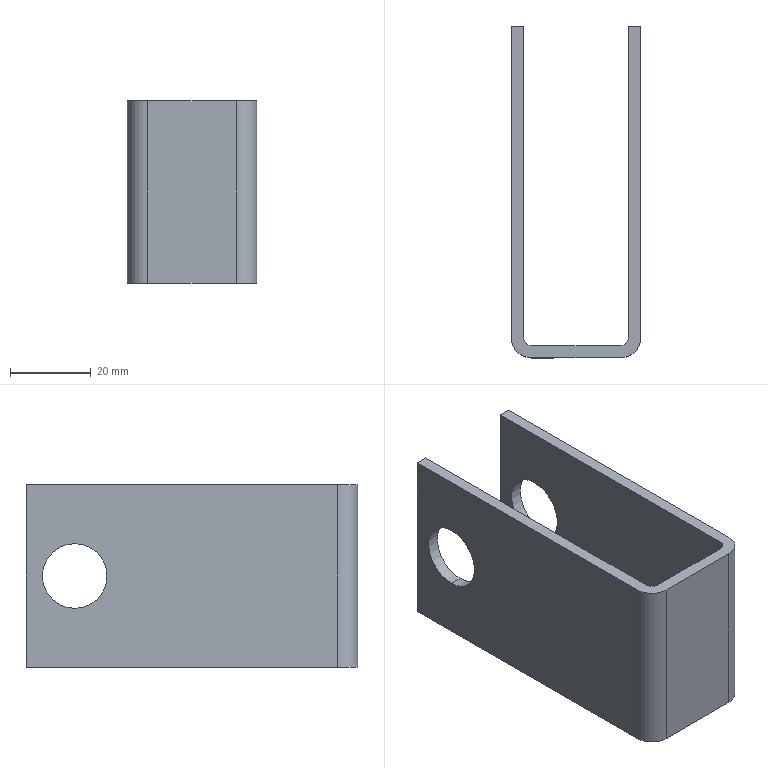Part | SolidWorks | features Extrusion 1, ICE 1 | 1 solid | 18 faces | box 32 x 82 x 45 mm | volume 24038 mm3 | plane 10 | cylinder 8 | commonest cylinder face diameters 16 x4 4 x2 10 x2
STEP:
#1=CARTESIAN_POINT('',(29.,-12.,30.5));
#2=VERTEX_POINT('',#1);
#3=CARTESIAN_POINT('',(29.,-12.,14.5));
#4=VERTEX_POINT('',#3);
#5=CARTESIAN_POINT('',(29.,-12.,22.5));
#6=DIRECTION('',(1.,0.,0.));
#7=DIRECTION('',(0.,1.,0.));
#8=AXIS2_PLACEMENT_3D('',#5,#6,#7);
#9=CIRCLE('',#8,8.);
#10=EDGE_CURVE('',#2,#4,#9,.T.);
#11=ORIENTED_EDGE('',*,*,#10,.F.);
#12=CARTESIAN_POINT('',(32.,-12.,30.5));
#13=VERTEX_POINT('',#12);
#14=CARTESIAN_POINT('',(0.,-12.,30.5));
#15=DIRECTION('',(1.,0.,0.));
#16=VECTOR('',#15,1000.);
#17=LINE('',#14,#16);
#18=EDGE_CURVE('',#2,#13,#17,.T.);
#19=ORIENTED_EDGE('',*,*,#18,.T.);
#20=CARTESIAN_POINT('',(32.,-12.,14.5));
#21=VERTEX_POINT('',#20);
#22=CARTESIAN_POINT('',(32.,-12.,22.5));
#23=DIRECTION('',(1.,0.,0.));
#24=DIRECTION('',(0.,0.,-1.));
#25=AXIS2_PLACEMENT_3D('',#22,#23,#24);
#26=CIRCLE('',#25,8.);
#27=EDGE_CURVE('',#13,#21,#26,.T.);
#28=ORIENTED_EDGE('',*,*,#27,.T.);
#29=CARTESIAN_POINT('',(0.,-12.,14.5));
#30=DIRECTION('',(1.,0.,0.));
#31=VECTOR('',#30,1000.);
#32=LINE('',#29,#31);
#33=EDGE_CURVE('',#4,#21,#32,.T.);
#34=ORIENTED_EDGE('',*,*,#33,.F.);
#35=EDGE_LOOP('',(#11,#19,#28,#34));
#36=FACE_OUTER_BOUND('',#35,.T.);
#37=CARTESIAN_POINT('',(0.,-12.,22.5));
#38=DIRECTION('',(1.,0.,0.));
#39=DIRECTION('',(0.,0.,-1.));
#40=AXIS2_PLACEMENT_3D('',#37,#38,#39);
#41=CYLINDRICAL_SURFACE('',#40,8.);
#42=ADVANCED_FACE('',(#36),#41,.F.);
#43=CARTESIAN_POINT('',(0.,-12.,30.5));
#44=VERTEX_POINT('',#43);
#45=CARTESIAN_POINT('',(0.,-12.,14.5));
#46=VERTEX_POINT('',#45);
#47=CARTESIAN_POINT('',(0.,-12.,22.5));
#48=DIRECTION('',(1.,0.,0.));
#49=DIRECTION('',(0.,0.,-1.));
#50=AXIS2_PLACEMENT_3D('',#47,#48,#49);
#51=CIRCLE('',#50,8.);
#52=EDGE_CURVE('',#44,#46,#51,.T.);
#53=ORIENTED_EDGE('',*,*,#52,.F.);
#54=CARTESIAN_POINT('',(3.,-12.,30.5));
#55=VERTEX_POINT('',#54);
#56=CARTESIAN_POINT('',(0.,-12.,30.5));
#57=DIRECTION('',(1.,0.,0.));
#58=VECTOR('',#57,1000.);
#59=LINE('',#56,#58);
#60=EDGE_CURVE('',#44,#55,#59,.T.);
#61=ORIENTED_EDGE('',*,*,#60,.T.);
#62=CARTESIAN_POINT('',(3.,-12.,14.5));
#63=VERTEX_POINT('',#62);
#64=CARTESIAN_POINT('',(3.,-12.,22.5));
#65=DIRECTION('',(-1.,0.,0.));
#66=DIRECTION('',(0.,-1.,0.));
#67=AXIS2_PLACEMENT_3D('',#64,#65,#66);
#68=CIRCLE('',#67,8.);
#69=EDGE_CURVE('',#63,#55,#68,.T.);
#70=ORIENTED_EDGE('',*,*,#69,.F.);
#71=CARTESIAN_POINT('',(0.,-12.,14.5));
#72=DIRECTION('',(1.,0.,0.));
#73=VECTOR('',#72,1000.);
#74=LINE('',#71,#73);
#75=EDGE_CURVE('',#46,#63,#74,.T.);
#76=ORIENTED_EDGE('',*,*,#75,.F.);
#77=EDGE_LOOP('',(#53,#61,#70,#76));
#78=FACE_OUTER_BOUND('',#77,.T.);
#79=CARTESIAN_POINT('',(0.,-12.,22.5));
#80=DIRECTION('',(1.,0.,0.));
#81=DIRECTION('',(0.,0.,-1.));
#82=AXIS2_PLACEMENT_3D('',#79,#80,#81);
#83=CYLINDRICAL_SURFACE('',#82,8.);
#84=ADVANCED_FACE('',(#78),#83,.F.);
#85=CARTESIAN_POINT('',(3.,0.,0.));
#86=VERTEX_POINT('',#85);
#87=CARTESIAN_POINT('',(0.,0.,0.));
#88=VERTEX_POINT('',#87);
#89=CARTESIAN_POINT('',(3.,0.,0.));
#90=DIRECTION('',(-1.,0.,0.));
#91=VECTOR('',#90,1000.);
#92=LINE('',#89,#91);
#93=EDGE_CURVE('',#86,#88,#92,.T.);
#94=ORIENTED_EDGE('',*,*,#93,.T.);
#95=CARTESIAN_POINT('',(0.,0.,45.));
#96=VERTEX_POINT('',#95);
#97=CARTESIAN_POINT('',(0.,0.,45.));
#98=DIRECTION('',(0.,0.,-1.));
#99=VECTOR('',#98,1000.);
#100=LINE('',#97,#99);
#101=EDGE_CURVE('',#96,#88,#100,.T.);
#102=ORIENTED_EDGE('',*,*,#101,.F.);
#103=CARTESIAN_POINT('',(3.,0.,45.));
#104=VERTEX_POINT('',#103);
#105=CARTESIAN_POINT('',(3.,0.,45.));
#106=DIRECTION('',(-1.,0.,0.));
#107=VECTOR('',#106,1000.);
#108=LINE('',#105,#107);
#109=EDGE_CURVE('',#104,#96,#108,.T.);
#110=ORIENTED_EDGE('',*,*,#109,.F.);
#111=CARTESIAN_POINT('',(3.,0.,45.));
#112=DIRECTION('',(0.,0.,-1.));
#113=VECTOR('',#112,1000.);
#114=LINE('',#111,#113);
#115=EDGE_CURVE('',#104,#86,#114,.T.);
#116=ORIENTED_EDGE('',*,*,#115,.T.);
#117=EDGE_LOOP('',(#94,#102,#110,#116));
#118=FACE_OUTER_BOUND('',#117,.T.);
#119=CARTESIAN_POINT('',(3.,0.,45.));
#120=DIRECTION('',(0.,-1.,0.));
#121=DIRECTION('',(0.,0.,-1.));
#122=AXIS2_PLACEMENT_3D('',#119,#120,#121);
#123=PLANE('',#122);
#124=ADVANCED_FACE('',(#118),#123,.F.);
#125=CARTESIAN_POINT('',(0.,-12.,22.5));
#126=DIRECTION('',(1.,0.,0.));
#127=DIRECTION('',(0.,0.,-1.));
#128=AXIS2_PLACEMENT_3D('',#125,#126,#127);
#129=CIRCLE('',#128,8.);
#130=EDGE_CURVE('',#46,#44,#129,.T.);
#131=ORIENTED_EDGE('',*,*,#130,.T.);
#132=ORIENTED_EDGE('',*,*,#52,.T.);
#133=EDGE_LOOP('',(#131,#132));
#134=FACE_BOUND('',#133,.T.);
#135=CARTESIAN_POINT('',(0.,-77.,0.));
#136=VERTEX_POINT('',#135);
#137=CARTESIAN_POINT('',(0.,0.,0.));
#138=DIRECTION('',(0.,-1.,0.));
#139=VECTOR('',#138,1000.);
#140=LINE('',#137,#139);
#141=EDGE_CURVE('',#88,#136,#140,.T.);
#142=ORIENTED_EDGE('',*,*,#141,.T.);
#143=CARTESIAN_POINT('',(0.,-77.,45.));
#144=VERTEX_POINT('',#143);
#145=CARTESIAN_POINT('',(0.,-77.,45.));
#146=DIRECTION('',(0.,0.,-1.));
#147=VECTOR('',#146,1000.);
#148=LINE('',#145,#147);
#149=EDGE_CURVE('',#144,#136,#148,.T.);
#150=ORIENTED_EDGE('',*,*,#149,.F.);
#151=CARTESIAN_POINT('',(0.,0.,45.));
#152=DIRECTION('',(0.,-1.,0.));
#153=VECTOR('',#152,1000.);
#154=LINE('',#151,#153);
#155=EDGE_CURVE('',#96,#144,#154,.T.);
#156=ORIENTED_EDGE('',*,*,#155,.F.);
#157=ORIENTED_EDGE('',*,*,#101,.T.);
#158=EDGE_LOOP('',(#142,#150,#156,#157));
#159=FACE_OUTER_BOUND('',#158,.T.);
#160=CARTESIAN_POINT('',(0.,0.,45.));
#161=DIRECTION('',(1.,0.,0.));
#162=DIRECTION('',(0.,1.,0.));
#163=AXIS2_PLACEMENT_3D('',#160,#161,#162);
#164=PLANE('',#163);
#165=ADVANCED_FACE('',(#134,#159),#164,.F.);
#166=CARTESIAN_POINT('',(5.,-82.,0.));
#167=VERTEX_POINT('',#166);
#168=CARTESIAN_POINT('',(5.,-77.,0.));
#169=DIRECTION('',(0.,0.,1.));
#170=DIRECTION('',(1.,0.,0.));
#171=AXIS2_PLACEMENT_3D('',#168,#169,#170);
#172=CIRCLE('',#171,5.);
#173=EDGE_CURVE('',#136,#167,#172,.T.);
#174=ORIENTED_EDGE('',*,*,#173,.T.);
#175=CARTESIAN_POINT('',(5.,-82.,45.));
#176=VERTEX_POINT('',#175);
#177=CARTESIAN_POINT('',(5.,-82.,45.));
#178=DIRECTION('',(0.,0.,-1.));
#179=VECTOR('',#178,1000.);
#180=LINE('',#177,#179);
#181=EDGE_CURVE('',#176,#167,#180,.T.);
#182=ORIENTED_EDGE('',*,*,#181,.F.);
#183=CARTESIAN_POINT('',(5.,-77.,45.));
#184=DIRECTION('',(0.,0.,1.));
#185=DIRECTION('',(1.,0.,0.));
#186=AXIS2_PLACEMENT_3D('',#183,#184,#185);
#187=CIRCLE('',#186,5.);
#188=EDGE_CURVE('',#144,#176,#187,.T.);
#189=ORIENTED_EDGE('',*,*,#188,.F.);
#190=ORIENTED_EDGE('',*,*,#149,.T.);
#191=EDGE_LOOP('',(#174,#182,#189,#190));
#192=FACE_OUTER_BOUND('',#191,.T.);
#193=CARTESIAN_POINT('',(5.,-77.,45.));
#194=DIRECTION('',(0.,0.,-1.));
#195=DIRECTION('',(-1.,0.,0.));
#196=AXIS2_PLACEMENT_3D('',#193,#194,#195);
#197=CYLINDRICAL_SURFACE('',#196,5.);
#198=ADVANCED_FACE('',(#192),#197,.T.);
#199=CARTESIAN_POINT('',(27.,-82.,0.));
#200=VERTEX_POINT('',#199);
#201=CARTESIAN_POINT('',(5.,-82.,0.));
#202=DIRECTION('',(1.,0.,0.));
#203=VECTOR('',#202,1000.);
#204=LINE('',#201,#203);
#205=EDGE_CURVE('',#167,#200,#204,.T.);
#206=ORIENTED_EDGE('',*,*,#205,.T.);
#207=CARTESIAN_POINT('',(27.,-82.,45.));
#208=VERTEX_POINT('',#207);
#209=CARTESIAN_POINT('',(27.,-82.,45.));
#210=DIRECTION('',(0.,0.,-1.));
#211=VECTOR('',#210,1000.);
#212=LINE('',#209,#211);
#213=EDGE_CURVE('',#208,#200,#212,.T.);
#214=ORIENTED_EDGE('',*,*,#213,.F.);
#215=CARTESIAN_POINT('',(5.,-82.,45.));
#216=DIRECTION('',(1.,0.,0.));
#217=VECTOR('',#216,1000.);
#218=LINE('',#215,#217);
#219=EDGE_CURVE('',#176,#208,#218,.T.);
#220=ORIENTED_EDGE('',*,*,#219,.F.);
#221=ORIENTED_EDGE('',*,*,#181,.T.);
#222=EDGE_LOOP('',(#206,#214,#220,#221));
#223=FACE_OUTER_BOUND('',#222,.T.);
#224=CARTESIAN_POINT('',(5.,-82.,45.));
#225=DIRECTION('',(0.,1.,0.));
#226=DIRECTION('',(-1.,0.,0.));
#227=AXIS2_PLACEMENT_3D('',#224,#225,#226);
#228=PLANE('',#227);
#229=ADVANCED_FACE('',(#223),#228,.F.);
#230=CARTESIAN_POINT('',(32.,-77.,0.));
#231=VERTEX_POINT('',#230);
#232=CARTESIAN_POINT('',(27.,-77.,0.));
#233=DIRECTION('',(0.,0.,1.));
#234=DIRECTION('',(1.,0.,0.));
#235=AXIS2_PLACEMENT_3D('',#232,#233,#234);
#236=CIRCLE('',#235,5.);
#237=EDGE_CURVE('',#200,#231,#236,.T.);
#238=ORIENTED_EDGE('',*,*,#237,.T.);
#239=CARTESIAN_POINT('',(32.,-77.,45.));
#240=VERTEX_POINT('',#239);
#241=CARTESIAN_POINT('',(32.,-77.,45.));
#242=DIRECTION('',(0.,0.,-1.));
#243=VECTOR('',#242,1000.);
#244=LINE('',#241,#243);
#245=EDGE_CURVE('',#240,#231,#244,.T.);
#246=ORIENTED_EDGE('',*,*,#245,.F.);
#247=CARTESIAN_POINT('',(27.,-77.,45.));
#248=DIRECTION('',(0.,0.,1.));
#249=DIRECTION('',(1.,0.,0.));
#250=AXIS2_PLACEMENT_3D('',#247,#248,#249);
#251=CIRCLE('',#250,5.);
#252=EDGE_CURVE('',#208,#240,#251,.T.);
#253=ORIENTED_EDGE('',*,*,#252,.F.);
#254=ORIENTED_EDGE('',*,*,#213,.T.);
#255=EDGE_LOOP('',(#238,#246,#253,#254));
#256=FACE_OUTER_BOUND('',#255,.T.);
#257=CARTESIAN_POINT('',(27.,-77.,45.));
#258=DIRECTION('',(0.,0.,-1.));
#259=DIRECTION('',(-1.,0.,0.));
#260=AXIS2_PLACEMENT_3D('',#257,#258,#259);
#261=CYLINDRICAL_SURFACE('',#260,5.);
#262=ADVANCED_FACE('',(#256),#261,.T.);
#263=CARTESIAN_POINT('',(32.,-12.,22.5));
#264=DIRECTION('',(1.,0.,0.));
#265=DIRECTION('',(0.,0.,-1.));
#266=AXIS2_PLACEMENT_3D('',#263,#264,#265);
#267=CIRCLE('',#266,8.);
#268=EDGE_CURVE('',#21,#13,#267,.T.);
#269=ORIENTED_EDGE('',*,*,#268,.F.);
#270=ORIENTED_EDGE('',*,*,#27,.F.);
#271=EDGE_LOOP('',(#269,#270));
#272=FACE_BOUND('',#271,.T.);
#273=CARTESIAN_POINT('',(32.,0.,0.));
#274=VERTEX_POINT('',#273);
#275=CARTESIAN_POINT('',(32.,-77.,0.));
#276=DIRECTION('',(0.,1.,0.));
#277=VECTOR('',#276,1000.);
#278=LINE('',#275,#277);
#279=EDGE_CURVE('',#231,#274,#278,.T.);
#280=ORIENTED_EDGE('',*,*,#279,.T.);
#281=CARTESIAN_POINT('',(32.,0.,45.));
#282=VERTEX_POINT('',#281);
#283=CARTESIAN_POINT('',(32.,0.,45.));
#284=DIRECTION('',(0.,0.,-1.));
#285=VECTOR('',#284,1000.);
#286=LINE('',#283,#285);
#287=EDGE_CURVE('',#282,#274,#286,.T.);
#288=ORIENTED_EDGE('',*,*,#287,.F.);
#289=CARTESIAN_POINT('',(32.,-77.,45.));
#290=DIRECTION('',(0.,1.,0.));
#291=VECTOR('',#290,1000.);
#292=LINE('',#289,#291);
#293=EDGE_CURVE('',#240,#282,#292,.T.);
#294=ORIENTED_EDGE('',*,*,#293,.F.);
#295=ORIENTED_EDGE('',*,*,#245,.T.);
#296=EDGE_LOOP('',(#280,#288,#294,#295));
#297=FACE_OUTER_BOUND('',#296,.T.);
#298=CARTESIAN_POINT('',(32.,-77.,45.));
#299=DIRECTION('',(-1.,0.,0.));
#300=DIRECTION('',(0.,0.,1.));
#301=AXIS2_PLACEMENT_3D('',#298,#299,#300);
#302=PLANE('',#301);
#303=ADVANCED_FACE('',(#272,#297),#302,.F.);
#304=CARTESIAN_POINT('',(29.,0.,0.));
#305=VERTEX_POINT('',#304);
#306=CARTESIAN_POINT('',(29.,0.,0.));
#307=DIRECTION('',(-1.,0.,0.));
#308=VECTOR('',#307,1000.);
#309=LINE('',#306,#308);
#310=EDGE_CURVE('',#274,#305,#309,.T.);
#311=ORIENTED_EDGE('',*,*,#310,.T.);
#312=CARTESIAN_POINT('',(29.,0.,45.));
#313=VERTEX_POINT('',#312);
#314=CARTESIAN_POINT('',(29.,0.,45.));
#315=DIRECTION('',(0.,0.,-1.));
#316=VECTOR('',#315,1000.);
#317=LINE('',#314,#316);
#318=EDGE_CURVE('',#313,#305,#317,.T.);
#319=ORIENTED_EDGE('',*,*,#318,.F.);
#320=CARTESIAN_POINT('',(29.,0.,45.));
#321=DIRECTION('',(-1.,0.,0.));
#322=VECTOR('',#321,1000.);
#323=LINE('',#320,#322);
#324=EDGE_CURVE('',#282,#313,#323,.T.);
#325=ORIENTED_EDGE('',*,*,#324,.F.);
#326=ORIENTED_EDGE('',*,*,#287,.T.);
#327=EDGE_LOOP('',(#311,#319,#325,#326));
#328=FACE_OUTER_BOUND('',#327,.T.);
#329=CARTESIAN_POINT('',(29.,0.,45.));
#330=DIRECTION('',(0.,-1.,0.));
#331=DIRECTION('',(1.,0.,0.));
#332=AXIS2_PLACEMENT_3D('',#329,#330,#331);
#333=PLANE('',#332);
#334=ADVANCED_FACE('',(#328),#333,.F.);
#335=CARTESIAN_POINT('',(29.,-12.,22.5));
#336=DIRECTION('',(1.,0.,0.));
#337=DIRECTION('',(0.,1.,0.));
#338=AXIS2_PLACEMENT_3D('',#335,#336,#337);
#339=CIRCLE('',#338,8.);
#340=EDGE_CURVE('',#4,#2,#339,.T.);
#341=ORIENTED_EDGE('',*,*,#340,.T.);
#342=ORIENTED_EDGE('',*,*,#10,.T.);
#343=EDGE_LOOP('',(#341,#342));
#344=FACE_BOUND('',#343,.T.);
#345=CARTESIAN_POINT('',(29.,-77.,0.));
#346=VERTEX_POINT('',#345);
#347=CARTESIAN_POINT('',(29.,-77.,0.));
#348=DIRECTION('',(0.,-1.,0.));
#349=VECTOR('',#348,1000.);
#350=LINE('',#347,#349);
#351=EDGE_CURVE('',#305,#346,#350,.T.);
#352=ORIENTED_EDGE('',*,*,#351,.T.);
#353=CARTESIAN_POINT('',(29.,-77.,45.));
#354=VERTEX_POINT('',#353);
#355=CARTESIAN_POINT('',(29.,-77.,45.));
#356=DIRECTION('',(0.,0.,-1.));
#357=VECTOR('',#356,1000.);
#358=LINE('',#355,#357);
#359=EDGE_CURVE('',#354,#346,#358,.T.);
#360=ORIENTED_EDGE('',*,*,#359,.F.);
#361=CARTESIAN_POINT('',(29.,-77.,45.));
#362=DIRECTION('',(0.,-1.,0.));
#363=VECTOR('',#362,1000.);
#364=LINE('',#361,#363);
#365=EDGE_CURVE('',#313,#354,#364,.T.);
#366=ORIENTED_EDGE('',*,*,#365,.F.);
#367=ORIENTED_EDGE('',*,*,#318,.T.);
#368=EDGE_LOOP('',(#352,#360,#366,#367));
#369=FACE_OUTER_BOUND('',#368,.T.);
#370=CARTESIAN_POINT('',(29.,-77.,45.));
#371=DIRECTION('',(1.,0.,0.));
#372=DIRECTION('',(0.,1.,0.));
#373=AXIS2_PLACEMENT_3D('',#370,#371,#372);
#374=PLANE('',#373);
#375=ADVANCED_FACE('',(#344,#369),#374,.F.);
#376=CARTESIAN_POINT('',(27.,-79.,0.));
#377=VERTEX_POINT('',#376);
#378=CARTESIAN_POINT('',(27.,-77.,0.));
#379=DIRECTION('',(0.,0.,-1.));
#380=DIRECTION('',(1.,0.,0.));
#381=AXIS2_PLACEMENT_3D('',#378,#379,#380);
#382=CIRCLE('',#381,2.);
#383=EDGE_CURVE('',#346,#377,#382,.T.);
#384=ORIENTED_EDGE('',*,*,#383,.T.);
#385=CARTESIAN_POINT('',(27.,-79.,45.));
#386=VERTEX_POINT('',#385);
#387=CARTESIAN_POINT('',(27.,-79.,45.));
#388=DIRECTION('',(0.,0.,-1.));
#389=VECTOR('',#388,1000.);
#390=LINE('',#387,#389);
#391=EDGE_CURVE('',#386,#377,#390,.T.);
#392=ORIENTED_EDGE('',*,*,#391,.F.);
#393=CARTESIAN_POINT('',(27.,-77.,45.));
#394=DIRECTION('',(0.,0.,-1.));
#395=DIRECTION('',(1.,0.,0.));
#396=AXIS2_PLACEMENT_3D('',#393,#394,#395);
#397=CIRCLE('',#396,2.);
#398=EDGE_CURVE('',#354,#386,#397,.T.);
#399=ORIENTED_EDGE('',*,*,#398,.F.);
#400=ORIENTED_EDGE('',*,*,#359,.T.);
#401=EDGE_LOOP('',(#384,#392,#399,#400));
#402=FACE_OUTER_BOUND('',#401,.T.);
#403=CARTESIAN_POINT('',(27.,-77.,45.));
#404=DIRECTION('',(0.,0.,-1.));
#405=DIRECTION('',(-1.,0.,0.));
#406=AXIS2_PLACEMENT_3D('',#403,#404,#405);
#407=CYLINDRICAL_SURFACE('',#406,2.);
#408=ADVANCED_FACE('',(#402),#407,.F.);
#409=CARTESIAN_POINT('',(5.,-79.,0.));
#410=VERTEX_POINT('',#409);
#411=CARTESIAN_POINT('',(5.,-79.,0.));
#412=DIRECTION('',(-1.,0.,0.));
#413=VECTOR('',#412,1000.);
#414=LINE('',#411,#413);
#415=EDGE_CURVE('',#377,#410,#414,.T.);
#416=ORIENTED_EDGE('',*,*,#415,.T.);
#417=CARTESIAN_POINT('',(5.,-79.,45.));
#418=VERTEX_POINT('',#417);
#419=CARTESIAN_POINT('',(5.,-79.,45.));
#420=DIRECTION('',(0.,0.,-1.));
#421=VECTOR('',#420,1000.);
#422=LINE('',#419,#421);
#423=EDGE_CURVE('',#418,#410,#422,.T.);
#424=ORIENTED_EDGE('',*,*,#423,.F.);
#425=CARTESIAN_POINT('',(5.,-79.,45.));
#426=DIRECTION('',(-1.,0.,0.));
#427=VECTOR('',#426,1000.);
#428=LINE('',#425,#427);
#429=EDGE_CURVE('',#386,#418,#428,.T.);
#430=ORIENTED_EDGE('',*,*,#429,.F.);
#431=ORIENTED_EDGE('',*,*,#391,.T.);
#432=EDGE_LOOP('',(#416,#424,#430,#431));
#433=FACE_OUTER_BOUND('',#432,.T.);
#434=CARTESIAN_POINT('',(5.,-79.,45.));
#435=DIRECTION('',(0.,-1.,0.));
#436=DIRECTION('',(0.,0.,-1.));
#437=AXIS2_PLACEMENT_3D('',#434,#435,#436);
#438=PLANE('',#437);
#439=ADVANCED_FACE('',(#433),#438,.F.);
#440=CARTESIAN_POINT('',(3.,-77.,0.));
#441=VERTEX_POINT('',#440);
#442=CARTESIAN_POINT('',(5.,-77.,0.));
#443=DIRECTION('',(0.,0.,-1.));
#444=DIRECTION('',(1.,0.,0.));
#445=AXIS2_PLACEMENT_3D('',#442,#443,#444);
#446=CIRCLE('',#445,2.);
#447=EDGE_CURVE('',#410,#441,#446,.T.);
#448=ORIENTED_EDGE('',*,*,#447,.T.);
#449=CARTESIAN_POINT('',(3.,-77.,45.));
#450=VERTEX_POINT('',#449);
#451=CARTESIAN_POINT('',(3.,-77.,45.));
#452=DIRECTION('',(0.,0.,-1.));
#453=VECTOR('',#452,1000.);
#454=LINE('',#451,#453);
#455=EDGE_CURVE('',#450,#441,#454,.T.);
#456=ORIENTED_EDGE('',*,*,#455,.F.);
#457=CARTESIAN_POINT('',(5.,-77.,45.));
#458=DIRECTION('',(0.,0.,-1.));
#459=DIRECTION('',(1.,0.,0.));
#460=AXIS2_PLACEMENT_3D('',#457,#458,#459);
#461=CIRCLE('',#460,2.);
#462=EDGE_CURVE('',#418,#450,#461,.T.);
#463=ORIENTED_EDGE('',*,*,#462,.F.);
#464=ORIENTED_EDGE('',*,*,#423,.T.);
#465=EDGE_LOOP('',(#448,#456,#463,#464));
#466=FACE_OUTER_BOUND('',#465,.T.);
#467=CARTESIAN_POINT('',(5.,-77.,45.));
#468=DIRECTION('',(0.,0.,-1.));
#469=DIRECTION('',(-1.,0.,0.));
#470=AXIS2_PLACEMENT_3D('',#467,#468,#469);
#471=CYLINDRICAL_SURFACE('',#470,2.);
#472=ADVANCED_FACE('',(#466),#471,.F.);
#473=ORIENTED_EDGE('',*,*,#69,.T.);
#474=CARTESIAN_POINT('',(3.,-12.,22.5));
#475=DIRECTION('',(-1.,0.,0.));
#476=DIRECTION('',(0.,-1.,0.));
#477=AXIS2_PLACEMENT_3D('',#474,#475,#476);
#478=CIRCLE('',#477,8.);
#479=EDGE_CURVE('',#55,#63,#478,.T.);
#480=ORIENTED_EDGE('',*,*,#479,.T.);
#481=EDGE_LOOP('',(#473,#480));
#482=FACE_BOUND('',#481,.T.);
#483=CARTESIAN_POINT('',(3.,0.,0.));
#484=DIRECTION('',(0.,1.,0.));
#485=VECTOR('',#484,1000.);
#486=LINE('',#483,#485);
#487=EDGE_CURVE('',#441,#86,#486,.T.);
#488=ORIENTED_EDGE('',*,*,#487,.T.);
#489=ORIENTED_EDGE('',*,*,#115,.F.);
#490=CARTESIAN_POINT('',(3.,0.,45.));
#491=DIRECTION('',(0.,1.,0.));
#492=VECTOR('',#491,1000.);
#493=LINE('',#490,#492);
#494=EDGE_CURVE('',#450,#104,#493,.T.);
#495=ORIENTED_EDGE('',*,*,#494,.F.);
#496=ORIENTED_EDGE('',*,*,#455,.T.);
#497=EDGE_LOOP('',(#488,#489,#495,#496));
#498=FACE_OUTER_BOUND('',#497,.T.);
#499=CARTESIAN_POINT('',(3.,0.,45.));
#500=DIRECTION('',(-1.,0.,0.));
#501=DIRECTION('',(0.,-1.,0.));
#502=AXIS2_PLACEMENT_3D('',#499,#500,#501);
#503=PLANE('',#502);
#504=ADVANCED_FACE('',(#482,#498),#503,.F.);
#505=ORIENTED_EDGE('',*,*,#109,.T.);
#506=ORIENTED_EDGE('',*,*,#155,.T.);
#507=ORIENTED_EDGE('',*,*,#188,.T.);
#508=ORIENTED_EDGE('',*,*,#219,.T.);
#509=ORIENTED_EDGE('',*,*,#252,.T.);
#510=ORIENTED_EDGE('',*,*,#293,.T.);
#511=ORIENTED_EDGE('',*,*,#324,.T.);
#512=ORIENTED_EDGE('',*,*,#365,.T.);
#513=ORIENTED_EDGE('',*,*,#398,.T.);
#514=ORIENTED_EDGE('',*,*,#429,.T.);
#515=ORIENTED_EDGE('',*,*,#462,.T.);
#516=ORIENTED_EDGE('',*,*,#494,.T.);
#517=EDGE_LOOP('',(#505,#506,#507,#508,#509,#510,#511,#512,#513,#514,#515,#516));
#518=FACE_OUTER_BOUND('',#517,.T.);
#519=CARTESIAN_POINT('',(5.,-77.,45.));
#520=DIRECTION('',(0.,0.,1.));
#521=DIRECTION('',(1.,0.,0.));
#522=AXIS2_PLACEMENT_3D('',#519,#520,#521);
#523=PLANE('',#522);
#524=ADVANCED_FACE('',(#518),#523,.T.);
#525=ORIENTED_EDGE('',*,*,#93,.F.);
#526=ORIENTED_EDGE('',*,*,#487,.F.);
#527=ORIENTED_EDGE('',*,*,#447,.F.);
#528=ORIENTED_EDGE('',*,*,#415,.F.);
#529=ORIENTED_EDGE('',*,*,#383,.F.);
#530=ORIENTED_EDGE('',*,*,#351,.F.);
#531=ORIENTED_EDGE('',*,*,#310,.F.);
#532=ORIENTED_EDGE('',*,*,#279,.F.);
#533=ORIENTED_EDGE('',*,*,#237,.F.);
#534=ORIENTED_EDGE('',*,*,#205,.F.);
#535=ORIENTED_EDGE('',*,*,#173,.F.);
#536=ORIENTED_EDGE('',*,*,#141,.F.);
#537=EDGE_LOOP('',(#525,#526,#527,#528,#529,#530,#531,#532,#533,#534,#535,#536));
#538=FACE_OUTER_BOUND('',#537,.T.);
#539=CARTESIAN_POINT('',(5.,-77.,0.));
#540=DIRECTION('',(0.,0.,1.));
#541=DIRECTION('',(1.,0.,0.));
#542=AXIS2_PLACEMENT_3D('',#539,#540,#541);
#543=PLANE('',#542);
#544=ADVANCED_FACE('',(#538),#543,.F.);
#545=ORIENTED_EDGE('',*,*,#60,.F.);
#546=ORIENTED_EDGE('',*,*,#130,.F.);
#547=ORIENTED_EDGE('',*,*,#75,.T.);
#548=ORIENTED_EDGE('',*,*,#479,.F.);
#549=EDGE_LOOP('',(#545,#546,#547,#548));
#550=FACE_OUTER_BOUND('',#549,.T.);
#551=CARTESIAN_POINT('',(0.,-12.,22.5));
#552=DIRECTION('',(1.,0.,0.));
#553=DIRECTION('',(0.,0.,-1.));
#554=AXIS2_PLACEMENT_3D('',#551,#552,#553);
#555=CYLINDRICAL_SURFACE('',#554,8.);
#556=ADVANCED_FACE('',(#550),#555,.F.);
#557=ORIENTED_EDGE('',*,*,#18,.F.);
#558=ORIENTED_EDGE('',*,*,#340,.F.);
#559=ORIENTED_EDGE('',*,*,#33,.T.);
#560=ORIENTED_EDGE('',*,*,#268,.T.);
#561=EDGE_LOOP('',(#557,#558,#559,#560));
#562=FACE_OUTER_BOUND('',#561,.T.);
#563=CARTESIAN_POINT('',(0.,-12.,22.5));
#564=DIRECTION('',(1.,0.,0.));
#565=DIRECTION('',(0.,0.,-1.));
#566=AXIS2_PLACEMENT_3D('',#563,#564,#565);
#567=CYLINDRICAL_SURFACE('',#566,8.);
#568=ADVANCED_FACE('',(#562),#567,.F.);
#569=CLOSED_SHELL('',(#42,#84,#124,#165,#198,#229,#262,#303,#334,#375,#408,#439,#472,#504,#524,#544,#556,#568));
#570=MANIFOLD_SOLID_BREP('',#569);
#571=CARTESIAN_POINT('',(0.,0.,0.));
#572=DIRECTION('',(0.,0.,1.));
#573=DIRECTION('',(1.,0.,0.));
#574=AXIS2_PLACEMENT_3D('',#571,#572,#573);
#575=(LENGTH_UNIT()NAMED_UNIT(*)SI_UNIT(.MILLI.,.METRE.));
#576=UNCERTAINTY_MEASURE_WITH_UNIT(LENGTH_MEASURE(0.00001),#575,'','');
#577=(NAMED_UNIT(*)PLANE_ANGLE_UNIT()SI_UNIT($,.RADIAN.));
#578=(NAMED_UNIT(*)SI_UNIT($,.STERADIAN.)SOLID_ANGLE_UNIT());
#579=(GEOMETRIC_REPRESENTATION_CONTEXT(3)GLOBAL_UNCERTAINTY_ASSIGNED_CONTEXT((#576))GLOBAL_UNIT_ASSIGNED_CONTEXT((#575,#577,#578))REPRESENTATION_CONTEXT('',''));
#580=ADVANCED_BREP_SHAPE_REPRESENTATION('',(#570,#574),#579);